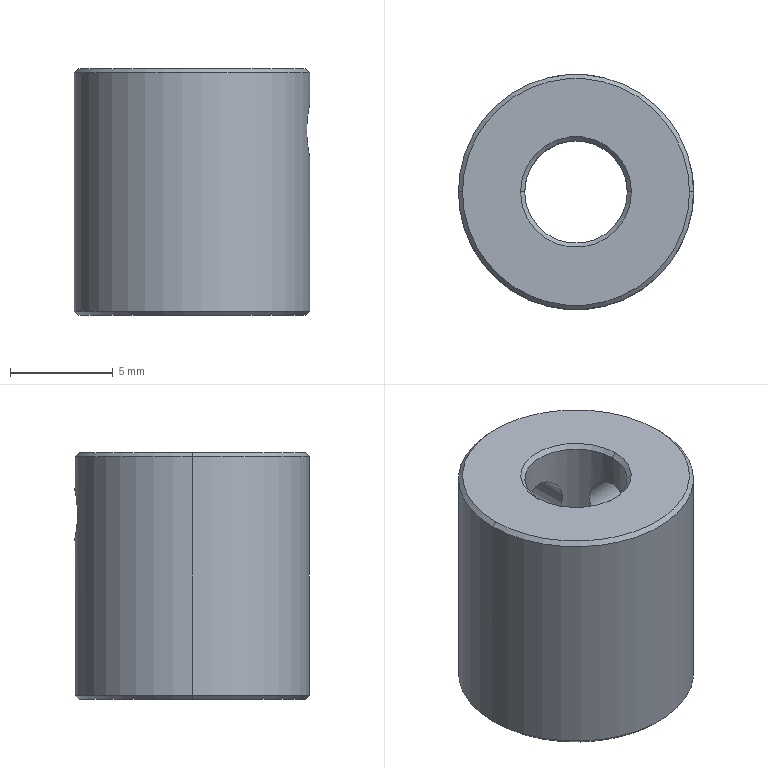Part | SolidWorks | features HoleWzd 2, Revolution 1 | 1 solid | 18 faces | box 11.46 x 11.46 x 12 mm | volume 967.917 mm3 | cylinder 8 | cone 8 | plane 2 | commonest cylinder face diameters 2.5 x4 5 x2 11.46 x2
STEP:
#1=CARTESIAN_POINT('',(5.73,0.,-1.75));
#2=VERTEX_POINT('',#1);
#3=CARTESIAN_POINT('',(5.73,0.,-4.25));
#4=VERTEX_POINT('',#3);
#5=CARTESIAN_POINT('',(5.73,0.,-1.75));
#6=CARTESIAN_POINT('',(5.73,-0.1657,-1.75));
#7=CARTESIAN_POINT('',(5.723,-0.3283,-1.783));
#8=CARTESIAN_POINT('',(5.697,-0.6308,-1.909));
#9=CARTESIAN_POINT('',(5.679,-0.7692,-2.001));
#10=CARTESIAN_POINT('',(5.643,-0.999,-2.231));
#11=CARTESIAN_POINT('',(5.625,-1.092,-2.37));
#12=CARTESIAN_POINT('',(5.6,-1.217,-2.671));
#13=CARTESIAN_POINT('',(5.592,-1.25,-2.836));
#14=CARTESIAN_POINT('',(5.592,-1.25,-3.081));
#15=CARTESIAN_POINT('',(5.594,-1.242,-3.164));
#16=CARTESIAN_POINT('',(5.601,-1.21,-3.325));
#17=CARTESIAN_POINT('',(5.606,-1.186,-3.403));
#18=CARTESIAN_POINT('',(5.625,-1.092,-3.63));
#19=CARTESIAN_POINT('',(5.643,-0.9998,-3.768));
#20=CARTESIAN_POINT('',(5.68,-0.7677,-4.));
#21=CARTESIAN_POINT('',(5.697,-0.63,-4.092));
#22=CARTESIAN_POINT('',(5.723,-0.3279,-4.217));
#23=CARTESIAN_POINT('',(5.73,-0.1634,-4.25));
#24=CARTESIAN_POINT('',(5.73,0.,-4.25));
#25=B_SPLINE_CURVE_WITH_KNOTS('',3,(#5,#6,#7,#8,#9,#10,#11,#12,#13,#14,#15,#16,#17,#18,#19,#20,#21,#22,#23,#24),.UNSPECIFIED.,.F.,.F.,(4,2,2,2,2,2,2,2,2,4),(0.,0.00049,0.00098,0.00147,0.00196,0.002205,0.00245,0.00294,0.00343,0.00392),.UNSPECIFIED.);
#26=EDGE_CURVE('',#2,#4,#25,.T.);
#27=ORIENTED_EDGE('',*,*,#26,.T.);
#28=CARTESIAN_POINT('',(2.5,0.,-4.25));
#29=VERTEX_POINT('',#28);
#30=CARTESIAN_POINT('',(0.,0.,-4.25));
#31=DIRECTION('',(-1.,0.,0.));
#32=VECTOR('',#31,1000.);
#33=LINE('',#30,#32);
#34=EDGE_CURVE('',#4,#29,#33,.T.);
#35=ORIENTED_EDGE('',*,*,#34,.T.);
#36=CARTESIAN_POINT('',(2.5,0.,-1.75));
#37=VERTEX_POINT('',#36);
#38=CARTESIAN_POINT('',(2.5,0.,-4.25));
#39=CARTESIAN_POINT('',(2.5,-0.08412,-4.25));
#40=CARTESIAN_POINT('',(2.496,-0.1666,-4.242));
#41=CARTESIAN_POINT('',(2.48,-0.3284,-4.209));
#42=CARTESIAN_POINT('',(2.468,-0.4085,-4.184));
#43=CARTESIAN_POINT('',(2.423,-0.635,-4.089));
#44=CARTESIAN_POINT('',(2.381,-0.7717,-3.996));
#45=CARTESIAN_POINT('',(2.295,-0.9981,-3.769));
#46=CARTESIAN_POINT('',(2.251,-1.09,-3.633));
#47=CARTESIAN_POINT('',(2.202,-1.184,-3.408));
#48=CARTESIAN_POINT('',(2.188,-1.209,-3.328));
#49=CARTESIAN_POINT('',(2.17,-1.242,-3.166));
#50=CARTESIAN_POINT('',(2.165,-1.25,-3.084));
#51=CARTESIAN_POINT('',(2.165,-1.25,-2.835));
#52=CARTESIAN_POINT('',(2.185,-1.216,-2.668));
#53=CARTESIAN_POINT('',(2.251,-1.089,-2.366));
#54=CARTESIAN_POINT('',(2.296,-0.9974,-2.23));
#55=CARTESIAN_POINT('',(2.381,-0.7706,-2.003));
#56=CARTESIAN_POINT('',(2.423,-0.6332,-1.91));
#57=CARTESIAN_POINT('',(2.482,-0.3331,-1.784));
#58=CARTESIAN_POINT('',(2.5,-0.166,-1.75));
#59=CARTESIAN_POINT('',(2.5,0.,-1.75));
#60=B_SPLINE_CURVE_WITH_KNOTS('',3,(#38,#39,#40,#41,#42,#43,#44,#45,#46,#47,#48,#49,#50,#51,#52,#53,#54,#55,#56,#57,#58,#59),.UNSPECIFIED.,.F.,.F.,(4,2,2,2,2,2,2,2,2,2,4),(0.,0.0002485,0.000497,0.0009941,0.001491,0.00174,0.001988,0.002485,0.002982,0.003479,0.003976),.UNSPECIFIED.);
#61=EDGE_CURVE('',#29,#37,#60,.T.);
#62=ORIENTED_EDGE('',*,*,#61,.T.);
#63=CARTESIAN_POINT('',(0.,0.,-1.75));
#64=DIRECTION('',(-1.,0.,0.));
#65=VECTOR('',#64,1000.);
#66=LINE('',#63,#65);
#67=EDGE_CURVE('',#2,#37,#66,.T.);
#68=ORIENTED_EDGE('',*,*,#67,.F.);
#69=EDGE_LOOP('',(#27,#35,#62,#68));
#70=FACE_OUTER_BOUND('',#69,.T.);
#71=CARTESIAN_POINT('',(0.,0.,-3.));
#72=DIRECTION('',(-1.,0.,0.));
#73=DIRECTION('',(0.,0.,1.));
#74=AXIS2_PLACEMENT_3D('',#71,#72,#73);
#75=CYLINDRICAL_SURFACE('',#74,1.25);
#76=ADVANCED_FACE('',(#70),#75,.F.);
#77=CARTESIAN_POINT('',(0.,5.73,-4.25));
#78=VERTEX_POINT('',#77);
#79=CARTESIAN_POINT('',(0.,5.73,-1.75));
#80=VERTEX_POINT('',#79);
#81=CARTESIAN_POINT('',(0.,5.73,-4.25));
#82=CARTESIAN_POINT('',(-0.1657,5.73,-4.25));
#83=CARTESIAN_POINT('',(-0.3283,5.723,-4.217));
#84=CARTESIAN_POINT('',(-0.6308,5.697,-4.091));
#85=CARTESIAN_POINT('',(-0.7692,5.679,-3.999));
#86=CARTESIAN_POINT('',(-0.999,5.643,-3.769));
#87=CARTESIAN_POINT('',(-1.092,5.625,-3.63));
#88=CARTESIAN_POINT('',(-1.217,5.6,-3.329));
#89=CARTESIAN_POINT('',(-1.25,5.592,-3.164));
#90=CARTESIAN_POINT('',(-1.25,5.592,-2.919));
#91=CARTESIAN_POINT('',(-1.242,5.594,-2.836));
#92=CARTESIAN_POINT('',(-1.21,5.601,-2.675));
#93=CARTESIAN_POINT('',(-1.186,5.606,-2.597));
#94=CARTESIAN_POINT('',(-1.092,5.625,-2.37));
#95=CARTESIAN_POINT('',(-0.9998,5.643,-2.232));
#96=CARTESIAN_POINT('',(-0.7677,5.68,-2.));
#97=CARTESIAN_POINT('',(-0.63,5.697,-1.908));
#98=CARTESIAN_POINT('',(-0.3279,5.723,-1.783));
#99=CARTESIAN_POINT('',(-0.1634,5.73,-1.75));
#100=CARTESIAN_POINT('',(0.,5.73,-1.75));
#101=B_SPLINE_CURVE_WITH_KNOTS('',3,(#81,#82,#83,#84,#85,#86,#87,#88,#89,#90,#91,#92,#93,#94,#95,#96,#97,#98,#99,#100),.UNSPECIFIED.,.F.,.F.,(4,2,2,2,2,2,2,2,2,4),(0.,0.00049,0.00098,0.00147,0.00196,0.002205,0.00245,0.00294,0.00343,0.00392),.UNSPECIFIED.);
#102=EDGE_CURVE('',#78,#80,#101,.T.);
#103=ORIENTED_EDGE('',*,*,#102,.T.);
#104=CARTESIAN_POINT('',(0.,2.5,-1.75));
#105=VERTEX_POINT('',#104);
#106=CARTESIAN_POINT('',(0.,0.,-1.75));
#107=DIRECTION('',(0.,-1.,0.));
#108=VECTOR('',#107,1000.);
#109=LINE('',#106,#108);
#110=EDGE_CURVE('',#80,#105,#109,.T.);
#111=ORIENTED_EDGE('',*,*,#110,.T.);
#112=CARTESIAN_POINT('',(0.,2.5,-4.25));
#113=VERTEX_POINT('',#112);
#114=CARTESIAN_POINT('',(0.,2.5,-1.75));
#115=CARTESIAN_POINT('',(-0.08285,2.5,-1.75));
#116=CARTESIAN_POINT('',(-0.1672,2.496,-1.758));
#117=CARTESIAN_POINT('',(-0.3292,2.48,-1.791));
#118=CARTESIAN_POINT('',(-0.4077,2.468,-1.815));
#119=CARTESIAN_POINT('',(-0.6361,2.423,-1.911));
#120=CARTESIAN_POINT('',(-0.7717,2.381,-2.004));
#121=CARTESIAN_POINT('',(-0.9986,2.295,-2.231));
#122=CARTESIAN_POINT('',(-1.09,2.251,-2.368));
#123=CARTESIAN_POINT('',(-1.216,2.186,-2.667));
#124=CARTESIAN_POINT('',(-1.25,2.165,-2.833));
#125=CARTESIAN_POINT('',(-1.25,2.165,-3.164));
#126=CARTESIAN_POINT('',(-1.217,2.185,-3.331));
#127=CARTESIAN_POINT('',(-1.09,2.251,-3.633));
#128=CARTESIAN_POINT('',(-0.9987,2.295,-3.769));
#129=CARTESIAN_POINT('',(-0.8277,2.36,-3.94));
#130=CARTESIAN_POINT('',(-0.7659,2.381,-3.991));
#131=CARTESIAN_POINT('',(-0.6321,2.42,-4.081));
#132=CARTESIAN_POINT('',(-0.5593,2.438,-4.121));
#133=CARTESIAN_POINT('',(-0.3335,2.482,-4.216));
#134=CARTESIAN_POINT('',(-0.168,2.5,-4.25));
#135=CARTESIAN_POINT('',(0.,2.5,-4.25));
#136=B_SPLINE_CURVE_WITH_KNOTS('',3,(#114,#115,#116,#117,#118,#119,#120,#121,#122,#123,#124,#125,#126,#127,#128,#129,#130,#131,#132,#133,#134,#135),.UNSPECIFIED.,.F.,.F.,(4,2,2,2,2,2,2,2,2,2,4),(0.003976,0.004224,0.004472,0.004969,0.005465,0.005961,0.006457,0.006953,0.007201,0.007449,0.007946),.UNSPECIFIED.);
#137=EDGE_CURVE('',#105,#113,#136,.T.);
#138=ORIENTED_EDGE('',*,*,#137,.T.);
#139=CARTESIAN_POINT('',(0.,0.,-4.25));
#140=DIRECTION('',(0.,-1.,0.));
#141=VECTOR('',#140,1000.);
#142=LINE('',#139,#141);
#143=EDGE_CURVE('',#78,#113,#142,.T.);
#144=ORIENTED_EDGE('',*,*,#143,.F.);
#145=EDGE_LOOP('',(#103,#111,#138,#144));
#146=FACE_OUTER_BOUND('',#145,.T.);
#147=CARTESIAN_POINT('',(0.,0.,-3.));
#148=DIRECTION('',(0.,-1.,0.));
#149=DIRECTION('',(0.,0.,-1.));
#150=AXIS2_PLACEMENT_3D('',#147,#148,#149);
#151=CYLINDRICAL_SURFACE('',#150,1.25);
#152=ADVANCED_FACE('',(#146),#151,.F.);
#153=CARTESIAN_POINT('',(-2.5,0.,-11.8));
#154=VERTEX_POINT('',#153);
#155=CARTESIAN_POINT('',(2.5,0.,-11.8));
#156=VERTEX_POINT('',#155);
#157=CARTESIAN_POINT('',(0.,0.,-11.8));
#158=DIRECTION('',(0.,0.,1.));
#159=DIRECTION('',(1.,0.,0.));
#160=AXIS2_PLACEMENT_3D('',#157,#158,#159);
#161=CIRCLE('',#160,2.5);
#162=EDGE_CURVE('',#154,#156,#161,.T.);
#163=ORIENTED_EDGE('',*,*,#162,.F.);
#164=CARTESIAN_POINT('',(-2.5,0.,-0.2));
#165=VERTEX_POINT('',#164);
#166=CARTESIAN_POINT('',(-2.5,0.,0.));
#167=DIRECTION('',(0.,0.,1.));
#168=VECTOR('',#167,1000.);
#169=LINE('',#166,#168);
#170=EDGE_CURVE('',#154,#165,#169,.T.);
#171=ORIENTED_EDGE('',*,*,#170,.T.);
#172=CARTESIAN_POINT('',(2.5,0.,-0.2));
#173=VERTEX_POINT('',#172);
#174=CARTESIAN_POINT('',(0.,0.,-0.2));
#175=DIRECTION('',(0.,0.,1.));
#176=DIRECTION('',(1.,0.,0.));
#177=AXIS2_PLACEMENT_3D('',#174,#175,#176);
#178=CIRCLE('',#177,2.5);
#179=EDGE_CURVE('',#165,#173,#178,.T.);
#180=ORIENTED_EDGE('',*,*,#179,.T.);
#181=CARTESIAN_POINT('',(2.5,0.,0.));
#182=DIRECTION('',(0.,0.,1.));
#183=VECTOR('',#182,1000.);
#184=LINE('',#181,#183);
#185=EDGE_CURVE('',#37,#173,#184,.T.);
#186=ORIENTED_EDGE('',*,*,#185,.F.);
#187=ORIENTED_EDGE('',*,*,#61,.F.);
#188=CARTESIAN_POINT('',(2.5,0.,0.));
#189=DIRECTION('',(0.,0.,1.));
#190=VECTOR('',#189,1000.);
#191=LINE('',#188,#190);
#192=EDGE_CURVE('',#156,#29,#191,.T.);
#193=ORIENTED_EDGE('',*,*,#192,.F.);
#194=EDGE_LOOP('',(#163,#171,#180,#186,#187,#193));
#195=FACE_OUTER_BOUND('',#194,.T.);
#196=CARTESIAN_POINT('',(0.,0.,0.));
#197=DIRECTION('',(0.,0.,1.));
#198=DIRECTION('',(1.,0.,0.));
#199=AXIS2_PLACEMENT_3D('',#196,#197,#198);
#200=CYLINDRICAL_SURFACE('',#199,2.5);
#201=ADVANCED_FACE('',(#195),#200,.F.);
#202=ORIENTED_EDGE('',*,*,#179,.F.);
#203=CARTESIAN_POINT('',(-2.7,0.,0.));
#204=VERTEX_POINT('',#203);
#205=CARTESIAN_POINT('',(-2.5,0.,-0.2));
#206=DIRECTION('',(-0.7071,0.,0.7071));
#207=VECTOR('',#206,1000.);
#208=LINE('',#205,#207);
#209=EDGE_CURVE('',#165,#204,#208,.T.);
#210=ORIENTED_EDGE('',*,*,#209,.T.);
#211=CARTESIAN_POINT('',(2.7,0.,0.));
#212=VERTEX_POINT('',#211);
#213=CARTESIAN_POINT('',(0.,0.,0.));
#214=DIRECTION('',(0.,0.,1.));
#215=DIRECTION('',(1.,0.,0.));
#216=AXIS2_PLACEMENT_3D('',#213,#214,#215);
#217=CIRCLE('',#216,2.7);
#218=EDGE_CURVE('',#204,#212,#217,.T.);
#219=ORIENTED_EDGE('',*,*,#218,.T.);
#220=CARTESIAN_POINT('',(2.5,0.,-0.2));
#221=DIRECTION('',(0.7071,0.,0.7071));
#222=VECTOR('',#221,1000.);
#223=LINE('',#220,#222);
#224=EDGE_CURVE('',#173,#212,#223,.T.);
#225=ORIENTED_EDGE('',*,*,#224,.F.);
#226=EDGE_LOOP('',(#202,#210,#219,#225));
#227=FACE_OUTER_BOUND('',#226,.T.);
#228=CARTESIAN_POINT('',(0.,0.,-0.2));
#229=DIRECTION('',(0.,0.,1.));
#230=DIRECTION('',(1.,0.,0.));
#231=AXIS2_PLACEMENT_3D('',#228,#229,#230);
#232=CONICAL_SURFACE('',#231,2.5,0.7854);
#233=ADVANCED_FACE('',(#227),#232,.F.);
#234=CARTESIAN_POINT('',(5.53,0.,0.));
#235=VERTEX_POINT('',#234);
#236=CARTESIAN_POINT('',(-5.53,0.,0.));
#237=VERTEX_POINT('',#236);
#238=CARTESIAN_POINT('',(0.,0.,0.));
#239=DIRECTION('',(0.,0.,1.));
#240=DIRECTION('',(1.,0.,0.));
#241=AXIS2_PLACEMENT_3D('',#238,#239,#240);
#242=CIRCLE('',#241,5.53);
#243=EDGE_CURVE('',#235,#237,#242,.T.);
#244=ORIENTED_EDGE('',*,*,#243,.F.);
#245=CARTESIAN_POINT('',(5.73,0.,-0.2));
#246=VERTEX_POINT('',#245);
#247=CARTESIAN_POINT('',(5.53,0.,0.));
#248=DIRECTION('',(0.7071,0.,-0.7071));
#249=VECTOR('',#248,1000.);
#250=LINE('',#247,#249);
#251=EDGE_CURVE('',#235,#246,#250,.T.);
#252=ORIENTED_EDGE('',*,*,#251,.T.);
#253=CARTESIAN_POINT('',(-5.73,0.,-0.2));
#254=VERTEX_POINT('',#253);
#255=CARTESIAN_POINT('',(0.,0.,-0.2));
#256=DIRECTION('',(0.,0.,1.));
#257=DIRECTION('',(1.,0.,0.));
#258=AXIS2_PLACEMENT_3D('',#255,#256,#257);
#259=CIRCLE('',#258,5.73);
#260=EDGE_CURVE('',#246,#254,#259,.T.);
#261=ORIENTED_EDGE('',*,*,#260,.T.);
#262=CARTESIAN_POINT('',(-5.53,0.,0.));
#263=DIRECTION('',(-0.7071,0.,-0.7071));
#264=VECTOR('',#263,1000.);
#265=LINE('',#262,#264);
#266=EDGE_CURVE('',#237,#254,#265,.T.);
#267=ORIENTED_EDGE('',*,*,#266,.F.);
#268=EDGE_LOOP('',(#244,#252,#261,#267));
#269=FACE_OUTER_BOUND('',#268,.T.);
#270=CARTESIAN_POINT('',(0.,0.,0.));
#271=DIRECTION('',(0.,0.,-1.));
#272=DIRECTION('',(-1.,0.,0.));
#273=AXIS2_PLACEMENT_3D('',#270,#271,#272);
#274=CONICAL_SURFACE('',#273,5.53,0.7854);
#275=ADVANCED_FACE('',(#269),#274,.T.);
#276=ORIENTED_EDGE('',*,*,#102,.F.);
#277=CARTESIAN_POINT('',(0.,5.73,-1.75));
#278=CARTESIAN_POINT('',(0.1634,5.73,-1.75));
#279=CARTESIAN_POINT('',(0.3283,5.723,-1.783));
#280=CARTESIAN_POINT('',(0.6293,5.697,-1.908));
#281=CARTESIAN_POINT('',(0.7681,5.679,-2.));
#282=CARTESIAN_POINT('',(0.9987,5.644,-2.231));
#283=CARTESIAN_POINT('',(1.091,5.626,-2.368));
#284=CARTESIAN_POINT('',(1.217,5.6,-2.672));
#285=CARTESIAN_POINT('',(1.25,5.592,-2.834));
#286=CARTESIAN_POINT('',(1.25,5.592,-3.082));
#287=CARTESIAN_POINT('',(1.242,5.594,-3.163));
#288=CARTESIAN_POINT('',(1.21,5.601,-3.324));
#289=CARTESIAN_POINT('',(1.186,5.606,-3.403));
#290=CARTESIAN_POINT('',(1.092,5.625,-3.63));
#291=CARTESIAN_POINT('',(0.9992,5.643,-3.768));
#292=CARTESIAN_POINT('',(0.7697,5.679,-3.998));
#293=CARTESIAN_POINT('',(0.6307,5.697,-4.091));
#294=CARTESIAN_POINT('',(0.33,5.722,-4.217));
#295=CARTESIAN_POINT('',(0.1657,5.73,-4.25));
#296=CARTESIAN_POINT('',(0.,5.73,-4.25));
#297=B_SPLINE_CURVE_WITH_KNOTS('',3,(#277,#278,#279,#280,#281,#282,#283,#284,#285,#286,#287,#288,#289,#290,#291,#292,#293,#294,#295,#296),.UNSPECIFIED.,.F.,.F.,(4,2,2,2,2,2,2,2,2,4),(0.00392,0.00441,0.0049,0.005389,0.005879,0.006124,0.006369,0.006859,0.007349,0.007839),.UNSPECIFIED.);
#298=EDGE_CURVE('',#80,#78,#297,.T.);
#299=ORIENTED_EDGE('',*,*,#298,.F.);
#300=EDGE_LOOP('',(#276,#299));
#301=FACE_BOUND('',#300,.T.);
#302=CARTESIAN_POINT('',(5.73,0.,-11.8));
#303=VERTEX_POINT('',#302);
#304=CARTESIAN_POINT('',(-5.73,0.,-11.8));
#305=VERTEX_POINT('',#304);
#306=CARTESIAN_POINT('',(0.,0.,-11.8));
#307=DIRECTION('',(0.,0.,1.));
#308=DIRECTION('',(1.,0.,0.));
#309=AXIS2_PLACEMENT_3D('',#306,#307,#308);
#310=CIRCLE('',#309,5.73);
#311=EDGE_CURVE('',#303,#305,#310,.T.);
#312=ORIENTED_EDGE('',*,*,#311,.T.);
#313=CARTESIAN_POINT('',(-5.73,0.,0.));
#314=DIRECTION('',(0.,0.,1.));
#315=VECTOR('',#314,1000.);
#316=LINE('',#313,#315);
#317=EDGE_CURVE('',#305,#254,#316,.T.);
#318=ORIENTED_EDGE('',*,*,#317,.T.);
#319=ORIENTED_EDGE('',*,*,#260,.F.);
#320=CARTESIAN_POINT('',(5.73,0.,0.));
#321=DIRECTION('',(0.,0.,1.));
#322=VECTOR('',#321,1000.);
#323=LINE('',#320,#322);
#324=EDGE_CURVE('',#2,#246,#323,.T.);
#325=ORIENTED_EDGE('',*,*,#324,.F.);
#326=CARTESIAN_POINT('',(5.73,0.,-4.25));
#327=CARTESIAN_POINT('',(5.73,0.1634,-4.25));
#328=CARTESIAN_POINT('',(5.723,0.3283,-4.217));
#329=CARTESIAN_POINT('',(5.697,0.6293,-4.092));
#330=CARTESIAN_POINT('',(5.679,0.7681,-4.));
#331=CARTESIAN_POINT('',(5.644,0.9987,-3.769));
#332=CARTESIAN_POINT('',(5.626,1.091,-3.632));
#333=CARTESIAN_POINT('',(5.6,1.217,-3.328));
#334=CARTESIAN_POINT('',(5.592,1.25,-3.166));
#335=CARTESIAN_POINT('',(5.592,1.25,-2.918));
#336=CARTESIAN_POINT('',(5.594,1.242,-2.837));
#337=CARTESIAN_POINT('',(5.601,1.21,-2.676));
#338=CARTESIAN_POINT('',(5.606,1.186,-2.597));
#339=CARTESIAN_POINT('',(5.625,1.092,-2.37));
#340=CARTESIAN_POINT('',(5.643,0.9992,-2.232));
#341=CARTESIAN_POINT('',(5.679,0.7697,-2.002));
#342=CARTESIAN_POINT('',(5.697,0.6307,-1.909));
#343=CARTESIAN_POINT('',(5.722,0.33,-1.783));
#344=CARTESIAN_POINT('',(5.73,0.1657,-1.75));
#345=CARTESIAN_POINT('',(5.73,0.,-1.75));
#346=B_SPLINE_CURVE_WITH_KNOTS('',3,(#326,#327,#328,#329,#330,#331,#332,#333,#334,#335,#336,#337,#338,#339,#340,#341,#342,#343,#344,#345),.UNSPECIFIED.,.F.,.F.,(4,2,2,2,2,2,2,2,2,4),(0.00392,0.00441,0.0049,0.005389,0.005879,0.006124,0.006369,0.006859,0.007349,0.007839),.UNSPECIFIED.);
#347=EDGE_CURVE('',#4,#2,#346,.T.);
#348=ORIENTED_EDGE('',*,*,#347,.F.);
#349=CARTESIAN_POINT('',(5.73,0.,0.));
#350=DIRECTION('',(0.,0.,1.));
#351=VECTOR('',#350,1000.);
#352=LINE('',#349,#351);
#353=EDGE_CURVE('',#303,#4,#352,.T.);
#354=ORIENTED_EDGE('',*,*,#353,.F.);
#355=EDGE_LOOP('',(#312,#318,#319,#325,#348,#354));
#356=FACE_OUTER_BOUND('',#355,.T.);
#357=CARTESIAN_POINT('',(0.,0.,0.));
#358=DIRECTION('',(0.,0.,1.));
#359=DIRECTION('',(1.,0.,0.));
#360=AXIS2_PLACEMENT_3D('',#357,#358,#359);
#361=CYLINDRICAL_SURFACE('',#360,5.73);
#362=ADVANCED_FACE('',(#301,#356),#361,.T.);
#363=CARTESIAN_POINT('',(5.53,0.,-12.));
#364=VERTEX_POINT('',#363);
#365=CARTESIAN_POINT('',(-5.53,0.,-12.));
#366=VERTEX_POINT('',#365);
#367=CARTESIAN_POINT('',(0.,0.,-12.));
#368=DIRECTION('',(0.,0.,1.));
#369=DIRECTION('',(1.,0.,0.));
#370=AXIS2_PLACEMENT_3D('',#367,#368,#369);
#371=CIRCLE('',#370,5.53);
#372=EDGE_CURVE('',#364,#366,#371,.T.);
#373=ORIENTED_EDGE('',*,*,#372,.T.);
#374=CARTESIAN_POINT('',(-5.73,0.,-11.8));
#375=DIRECTION('',(-0.7071,0.,0.7071));
#376=VECTOR('',#375,1000.);
#377=LINE('',#374,#376);
#378=EDGE_CURVE('',#366,#305,#377,.T.);
#379=ORIENTED_EDGE('',*,*,#378,.T.);
#380=ORIENTED_EDGE('',*,*,#311,.F.);
#381=CARTESIAN_POINT('',(5.73,0.,-11.8));
#382=DIRECTION('',(0.7071,0.,0.7071));
#383=VECTOR('',#382,1000.);
#384=LINE('',#381,#383);
#385=EDGE_CURVE('',#364,#303,#384,.T.);
#386=ORIENTED_EDGE('',*,*,#385,.F.);
#387=EDGE_LOOP('',(#373,#379,#380,#386));
#388=FACE_OUTER_BOUND('',#387,.T.);
#389=CARTESIAN_POINT('',(0.,0.,-11.8));
#390=DIRECTION('',(0.,0.,1.));
#391=DIRECTION('',(1.,0.,0.));
#392=AXIS2_PLACEMENT_3D('',#389,#390,#391);
#393=CONICAL_SURFACE('',#392,5.73,0.7854);
#394=ADVANCED_FACE('',(#388),#393,.T.);
#395=ORIENTED_EDGE('',*,*,#162,.T.);
#396=CARTESIAN_POINT('',(2.7,0.,-12.));
#397=VERTEX_POINT('',#396);
#398=CARTESIAN_POINT('',(2.7,0.,-12.));
#399=DIRECTION('',(0.7071,0.,-0.7071));
#400=VECTOR('',#399,1000.);
#401=LINE('',#398,#400);
#402=EDGE_CURVE('',#156,#397,#401,.T.);
#403=ORIENTED_EDGE('',*,*,#402,.T.);
#404=CARTESIAN_POINT('',(-2.7,0.,-12.));
#405=VERTEX_POINT('',#404);
#406=CARTESIAN_POINT('',(0.,0.,-12.));
#407=DIRECTION('',(0.,0.,1.));
#408=DIRECTION('',(1.,0.,0.));
#409=AXIS2_PLACEMENT_3D('',#406,#407,#408);
#410=CIRCLE('',#409,2.7);
#411=EDGE_CURVE('',#405,#397,#410,.T.);
#412=ORIENTED_EDGE('',*,*,#411,.F.);
#413=CARTESIAN_POINT('',(-2.7,0.,-12.));
#414=DIRECTION('',(-0.7071,0.,-0.7071));
#415=VECTOR('',#414,1000.);
#416=LINE('',#413,#415);
#417=EDGE_CURVE('',#154,#405,#416,.T.);
#418=ORIENTED_EDGE('',*,*,#417,.F.);
#419=EDGE_LOOP('',(#395,#403,#412,#418));
#420=FACE_OUTER_BOUND('',#419,.T.);
#421=CARTESIAN_POINT('',(0.,0.,-12.));
#422=DIRECTION('',(0.,0.,-1.));
#423=DIRECTION('',(-1.,0.,0.));
#424=AXIS2_PLACEMENT_3D('',#421,#422,#423);
#425=CONICAL_SURFACE('',#424,2.7,0.7854);
#426=ADVANCED_FACE('',(#420),#425,.F.);
#427=ORIENTED_EDGE('',*,*,#402,.F.);
#428=CARTESIAN_POINT('',(0.,0.,-11.8));
#429=DIRECTION('',(0.,0.,1.));
#430=DIRECTION('',(1.,0.,0.));
#431=AXIS2_PLACEMENT_3D('',#428,#429,#430);
#432=CIRCLE('',#431,2.5);
#433=EDGE_CURVE('',#156,#154,#432,.T.);
#434=ORIENTED_EDGE('',*,*,#433,.T.);
#435=ORIENTED_EDGE('',*,*,#417,.T.);
#436=CARTESIAN_POINT('',(0.,0.,-12.));
#437=DIRECTION('',(0.,0.,1.));
#438=DIRECTION('',(1.,0.,0.));
#439=AXIS2_PLACEMENT_3D('',#436,#437,#438);
#440=CIRCLE('',#439,2.7);
#441=EDGE_CURVE('',#397,#405,#440,.T.);
#442=ORIENTED_EDGE('',*,*,#441,.F.);
#443=EDGE_LOOP('',(#427,#434,#435,#442));
#444=FACE_OUTER_BOUND('',#443,.T.);
#445=CARTESIAN_POINT('',(0.,0.,-12.));
#446=DIRECTION('',(0.,0.,-1.));
#447=DIRECTION('',(-1.,0.,0.));
#448=AXIS2_PLACEMENT_3D('',#445,#446,#447);
#449=CONICAL_SURFACE('',#448,2.7,0.7854);
#450=ADVANCED_FACE('',(#444),#449,.F.);
#451=ORIENTED_EDGE('',*,*,#411,.T.);
#452=ORIENTED_EDGE('',*,*,#441,.T.);
#453=EDGE_LOOP('',(#451,#452));
#454=FACE_BOUND('',#453,.T.);
#455=ORIENTED_EDGE('',*,*,#372,.F.);
#456=CARTESIAN_POINT('',(0.,0.,-12.));
#457=DIRECTION('',(0.,0.,1.));
#458=DIRECTION('',(1.,0.,0.));
#459=AXIS2_PLACEMENT_3D('',#456,#457,#458);
#460=CIRCLE('',#459,5.53);
#461=EDGE_CURVE('',#366,#364,#460,.T.);
#462=ORIENTED_EDGE('',*,*,#461,.F.);
#463=EDGE_LOOP('',(#455,#462));
#464=FACE_OUTER_BOUND('',#463,.T.);
#465=CARTESIAN_POINT('',(2.7,0.,-12.));
#466=DIRECTION('',(0.,0.,-1.));
#467=DIRECTION('',(-1.,0.,0.));
#468=AXIS2_PLACEMENT_3D('',#465,#466,#467);
#469=PLANE('',#468);
#470=ADVANCED_FACE('',(#454,#464),#469,.T.);
#471=ORIENTED_EDGE('',*,*,#378,.F.);
#472=ORIENTED_EDGE('',*,*,#461,.T.);
#473=ORIENTED_EDGE('',*,*,#385,.T.);
#474=CARTESIAN_POINT('',(0.,0.,-11.8));
#475=DIRECTION('',(0.,0.,1.));
#476=DIRECTION('',(1.,0.,0.));
#477=AXIS2_PLACEMENT_3D('',#474,#475,#476);
#478=CIRCLE('',#477,5.73);
#479=EDGE_CURVE('',#305,#303,#478,.T.);
#480=ORIENTED_EDGE('',*,*,#479,.F.);
#481=EDGE_LOOP('',(#471,#472,#473,#480));
#482=FACE_OUTER_BOUND('',#481,.T.);
#483=CARTESIAN_POINT('',(0.,0.,-11.8));
#484=DIRECTION('',(0.,0.,1.));
#485=DIRECTION('',(1.,0.,0.));
#486=AXIS2_PLACEMENT_3D('',#483,#484,#485);
#487=CONICAL_SURFACE('',#486,5.73,0.7854);
#488=ADVANCED_FACE('',(#482),#487,.T.);
#489=ORIENTED_EDGE('',*,*,#317,.F.);
#490=ORIENTED_EDGE('',*,*,#479,.T.);
#491=ORIENTED_EDGE('',*,*,#353,.T.);
#492=ORIENTED_EDGE('',*,*,#26,.F.);
#493=ORIENTED_EDGE('',*,*,#324,.T.);
#494=CARTESIAN_POINT('',(0.,0.,-0.2));
#495=DIRECTION('',(0.,0.,1.));
#496=DIRECTION('',(1.,0.,0.));
#497=AXIS2_PLACEMENT_3D('',#494,#495,#496);
#498=CIRCLE('',#497,5.73);
#499=EDGE_CURVE('',#254,#246,#498,.T.);
#500=ORIENTED_EDGE('',*,*,#499,.F.);
#501=EDGE_LOOP('',(#489,#490,#491,#492,#493,#500));
#502=FACE_OUTER_BOUND('',#501,.T.);
#503=CARTESIAN_POINT('',(0.,0.,0.));
#504=DIRECTION('',(0.,0.,1.));
#505=DIRECTION('',(1.,0.,0.));
#506=AXIS2_PLACEMENT_3D('',#503,#504,#505);
#507=CYLINDRICAL_SURFACE('',#506,5.73);
#508=ADVANCED_FACE('',(#502),#507,.T.);
#509=ORIENTED_EDGE('',*,*,#251,.F.);
#510=CARTESIAN_POINT('',(0.,0.,0.));
#511=DIRECTION('',(0.,0.,1.));
#512=DIRECTION('',(1.,0.,0.));
#513=AXIS2_PLACEMENT_3D('',#510,#511,#512);
#514=CIRCLE('',#513,5.53);
#515=EDGE_CURVE('',#237,#235,#514,.T.);
#516=ORIENTED_EDGE('',*,*,#515,.F.);
#517=ORIENTED_EDGE('',*,*,#266,.T.);
#518=ORIENTED_EDGE('',*,*,#499,.T.);
#519=EDGE_LOOP('',(#509,#516,#517,#518));
#520=FACE_OUTER_BOUND('',#519,.T.);
#521=CARTESIAN_POINT('',(0.,0.,0.));
#522=DIRECTION('',(0.,0.,-1.));
#523=DIRECTION('',(-1.,0.,0.));
#524=AXIS2_PLACEMENT_3D('',#521,#522,#523);
#525=CONICAL_SURFACE('',#524,5.53,0.7854);
#526=ADVANCED_FACE('',(#520),#525,.T.);
#527=ORIENTED_EDGE('',*,*,#515,.T.);
#528=ORIENTED_EDGE('',*,*,#243,.T.);
#529=EDGE_LOOP('',(#527,#528));
#530=FACE_OUTER_BOUND('',#529,.T.);
#531=CARTESIAN_POINT('',(0.,0.,0.));
#532=DIRECTION('',(0.,0.,1.));
#533=DIRECTION('',(1.,0.,0.));
#534=AXIS2_PLACEMENT_3D('',#531,#532,#533);
#535=CIRCLE('',#534,2.7);
#536=EDGE_CURVE('',#212,#204,#535,.T.);
#537=ORIENTED_EDGE('',*,*,#536,.F.);
#538=ORIENTED_EDGE('',*,*,#218,.F.);
#539=EDGE_LOOP('',(#537,#538));
#540=FACE_BOUND('',#539,.T.);
#541=CARTESIAN_POINT('',(2.7,0.,0.));
#542=DIRECTION('',(0.,0.,1.));
#543=DIRECTION('',(1.,0.,0.));
#544=AXIS2_PLACEMENT_3D('',#541,#542,#543);
#545=PLANE('',#544);
#546=ADVANCED_FACE('',(#530,#540),#545,.T.);
#547=ORIENTED_EDGE('',*,*,#209,.F.);
#548=CARTESIAN_POINT('',(0.,0.,-0.2));
#549=DIRECTION('',(0.,0.,1.));
#550=DIRECTION('',(1.,0.,0.));
#551=AXIS2_PLACEMENT_3D('',#548,#549,#550);
#552=CIRCLE('',#551,2.5);
#553=EDGE_CURVE('',#173,#165,#552,.T.);
#554=ORIENTED_EDGE('',*,*,#553,.F.);
#555=ORIENTED_EDGE('',*,*,#224,.T.);
#556=ORIENTED_EDGE('',*,*,#536,.T.);
#557=EDGE_LOOP('',(#547,#554,#555,#556));
#558=FACE_OUTER_BOUND('',#557,.T.);
#559=CARTESIAN_POINT('',(0.,0.,-0.2));
#560=DIRECTION('',(0.,0.,1.));
#561=DIRECTION('',(1.,0.,0.));
#562=AXIS2_PLACEMENT_3D('',#559,#560,#561);
#563=CONICAL_SURFACE('',#562,2.5,0.7854);
#564=ADVANCED_FACE('',(#558),#563,.F.);
#565=ORIENTED_EDGE('',*,*,#170,.F.);
#566=ORIENTED_EDGE('',*,*,#433,.F.);
#567=ORIENTED_EDGE('',*,*,#192,.T.);
#568=CARTESIAN_POINT('',(2.5,0.,-1.75));
#569=CARTESIAN_POINT('',(2.5,0.08285,-1.75));
#570=CARTESIAN_POINT('',(2.496,0.1672,-1.758));
#571=CARTESIAN_POINT('',(2.48,0.3292,-1.791));
#572=CARTESIAN_POINT('',(2.468,0.4077,-1.815));
#573=CARTESIAN_POINT('',(2.423,0.6361,-1.911));
#574=CARTESIAN_POINT('',(2.381,0.7717,-2.004));
#575=CARTESIAN_POINT('',(2.295,0.9986,-2.231));
#576=CARTESIAN_POINT('',(2.251,1.09,-2.368));
#577=CARTESIAN_POINT('',(2.186,1.216,-2.667));
#578=CARTESIAN_POINT('',(2.165,1.25,-2.833));
#579=CARTESIAN_POINT('',(2.165,1.25,-3.164));
#580=CARTESIAN_POINT('',(2.185,1.217,-3.331));
#581=CARTESIAN_POINT('',(2.251,1.09,-3.633));
#582=CARTESIAN_POINT('',(2.295,0.9987,-3.769));
#583=CARTESIAN_POINT('',(2.36,0.8277,-3.94));
#584=CARTESIAN_POINT('',(2.381,0.7659,-3.991));
#585=CARTESIAN_POINT('',(2.42,0.6321,-4.081));
#586=CARTESIAN_POINT('',(2.438,0.5593,-4.121));
#587=CARTESIAN_POINT('',(2.482,0.3335,-4.216));
#588=CARTESIAN_POINT('',(2.5,0.168,-4.25));
#589=CARTESIAN_POINT('',(2.5,0.,-4.25));
#590=B_SPLINE_CURVE_WITH_KNOTS('',3,(#568,#569,#570,#571,#572,#573,#574,#575,#576,#577,#578,#579,#580,#581,#582,#583,#584,#585,#586,#587,#588,#589),.UNSPECIFIED.,.F.,.F.,(4,2,2,2,2,2,2,2,2,2,4),(0.003976,0.004224,0.004472,0.004969,0.005465,0.005961,0.006457,0.006953,0.007201,0.007449,0.007946),.UNSPECIFIED.);
#591=EDGE_CURVE('',#37,#29,#590,.T.);
#592=ORIENTED_EDGE('',*,*,#591,.F.);
#593=ORIENTED_EDGE('',*,*,#185,.T.);
#594=ORIENTED_EDGE('',*,*,#553,.T.);
#595=EDGE_LOOP('',(#565,#566,#567,#592,#593,#594));
#596=FACE_OUTER_BOUND('',#595,.T.);
#597=CARTESIAN_POINT('',(0.,2.5,-4.25));
#598=CARTESIAN_POINT('',(0.08412,2.5,-4.25));
#599=CARTESIAN_POINT('',(0.1666,2.496,-4.242));
#600=CARTESIAN_POINT('',(0.3284,2.48,-4.209));
#601=CARTESIAN_POINT('',(0.4085,2.468,-4.184));
#602=CARTESIAN_POINT('',(0.635,2.423,-4.089));
#603=CARTESIAN_POINT('',(0.7717,2.381,-3.996));
#604=CARTESIAN_POINT('',(0.9981,2.295,-3.769));
#605=CARTESIAN_POINT('',(1.09,2.251,-3.633));
#606=CARTESIAN_POINT('',(1.184,2.202,-3.408));
#607=CARTESIAN_POINT('',(1.209,2.188,-3.328));
#608=CARTESIAN_POINT('',(1.242,2.17,-3.166));
#609=CARTESIAN_POINT('',(1.25,2.165,-3.084));
#610=CARTESIAN_POINT('',(1.25,2.165,-2.835));
#611=CARTESIAN_POINT('',(1.216,2.185,-2.668));
#612=CARTESIAN_POINT('',(1.089,2.251,-2.366));
#613=CARTESIAN_POINT('',(0.9974,2.296,-2.23));
#614=CARTESIAN_POINT('',(0.7706,2.381,-2.003));
#615=CARTESIAN_POINT('',(0.6332,2.423,-1.91));
#616=CARTESIAN_POINT('',(0.3331,2.482,-1.784));
#617=CARTESIAN_POINT('',(0.166,2.5,-1.75));
#618=CARTESIAN_POINT('',(0.,2.5,-1.75));
#619=B_SPLINE_CURVE_WITH_KNOTS('',3,(#597,#598,#599,#600,#601,#602,#603,#604,#605,#606,#607,#608,#609,#610,#611,#612,#613,#614,#615,#616,#617,#618),.UNSPECIFIED.,.F.,.F.,(4,2,2,2,2,2,2,2,2,2,4),(0.,0.0002485,0.000497,0.0009941,0.001491,0.00174,0.001988,0.002485,0.002982,0.003479,0.003976),.UNSPECIFIED.);
#620=EDGE_CURVE('',#113,#105,#619,.T.);
#621=ORIENTED_EDGE('',*,*,#620,.F.);
#622=ORIENTED_EDGE('',*,*,#137,.F.);
#623=EDGE_LOOP('',(#621,#622));
#624=FACE_BOUND('',#623,.T.);
#625=CARTESIAN_POINT('',(0.,0.,0.));
#626=DIRECTION('',(0.,0.,1.));
#627=DIRECTION('',(1.,0.,0.));
#628=AXIS2_PLACEMENT_3D('',#625,#626,#627);
#629=CYLINDRICAL_SURFACE('',#628,2.5);
#630=ADVANCED_FACE('',(#596,#624),#629,.F.);
#631=ORIENTED_EDGE('',*,*,#110,.F.);
#632=ORIENTED_EDGE('',*,*,#298,.T.);
#633=ORIENTED_EDGE('',*,*,#143,.T.);
#634=ORIENTED_EDGE('',*,*,#620,.T.);
#635=EDGE_LOOP('',(#631,#632,#633,#634));
#636=FACE_OUTER_BOUND('',#635,.T.);
#637=CARTESIAN_POINT('',(0.,0.,-3.));
#638=DIRECTION('',(0.,-1.,0.));
#639=DIRECTION('',(0.,0.,-1.));
#640=AXIS2_PLACEMENT_3D('',#637,#638,#639);
#641=CYLINDRICAL_SURFACE('',#640,1.25);
#642=ADVANCED_FACE('',(#636),#641,.F.);
#643=ORIENTED_EDGE('',*,*,#34,.F.);
#644=ORIENTED_EDGE('',*,*,#347,.T.);
#645=ORIENTED_EDGE('',*,*,#67,.T.);
#646=ORIENTED_EDGE('',*,*,#591,.T.);
#647=EDGE_LOOP('',(#643,#644,#645,#646));
#648=FACE_OUTER_BOUND('',#647,.T.);
#649=CARTESIAN_POINT('',(0.,0.,-3.));
#650=DIRECTION('',(-1.,0.,0.));
#651=DIRECTION('',(0.,0.,1.));
#652=AXIS2_PLACEMENT_3D('',#649,#650,#651);
#653=CYLINDRICAL_SURFACE('',#652,1.25);
#654=ADVANCED_FACE('',(#648),#653,.F.);
#655=CLOSED_SHELL('',(#76,#152,#201,#233,#275,#362,#394,#426,#450,#470,#488,#508,#526,#546,#564,#630,#642,#654));
#656=MANIFOLD_SOLID_BREP('',#655);
#657=CARTESIAN_POINT('',(0.,0.,0.));
#658=DIRECTION('',(0.,0.,1.));
#659=DIRECTION('',(1.,0.,0.));
#660=AXIS2_PLACEMENT_3D('',#657,#658,#659);
#661=(LENGTH_UNIT()NAMED_UNIT(*)SI_UNIT(.MILLI.,.METRE.));
#662=UNCERTAINTY_MEASURE_WITH_UNIT(LENGTH_MEASURE(0.00001),#661,'','');
#663=(NAMED_UNIT(*)PLANE_ANGLE_UNIT()SI_UNIT($,.RADIAN.));
#664=(NAMED_UNIT(*)SI_UNIT($,.STERADIAN.)SOLID_ANGLE_UNIT());
#665=(GEOMETRIC_REPRESENTATION_CONTEXT(3)GLOBAL_UNCERTAINTY_ASSIGNED_CONTEXT((#662))GLOBAL_UNIT_ASSIGNED_CONTEXT((#661,#663,#664))REPRESENTATION_CONTEXT('',''));
#666=ADVANCED_BREP_SHAPE_REPRESENTATION('',(#656,#660),#665);